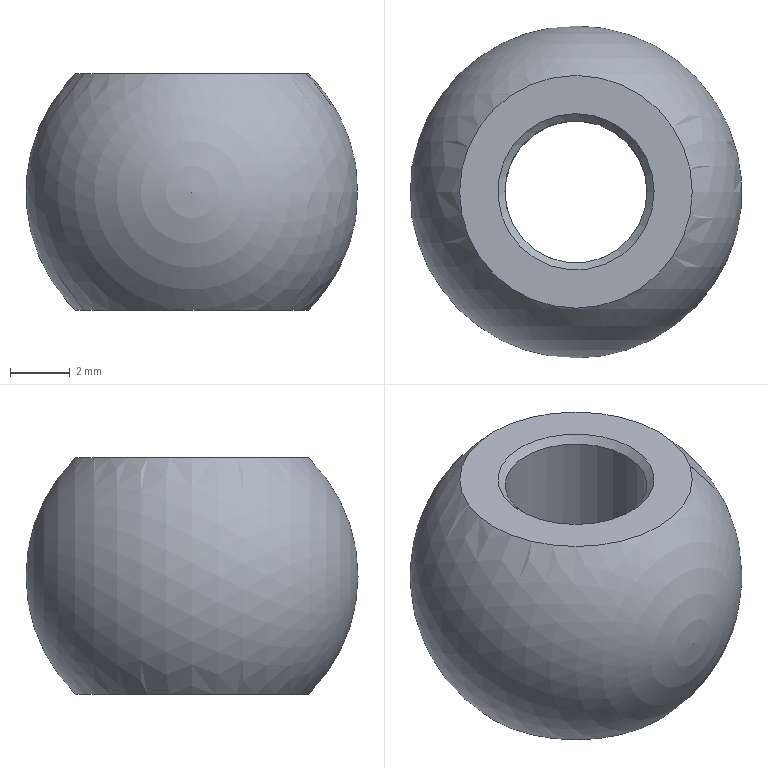Part | NX | features MG0312 tapped 1064K711(1064K711) 2 | 1 solid | 6 faces | box 11.125 x 11.125 x 7.938 mm | volume 498.388 mm3 | plane 2 | cone 2 | sphere 1 | cylinder 1 | commonest cylinder face diameters 4.763 x1
STEP:
#1=CARTESIAN_POINT('',(0.,10.39,-3.969));
#2=VERTEX_POINT('',#1);
#3=CARTESIAN_POINT('',(0.,14.287,-3.969));
#4=DIRECTION('',(0.,0.,1.));
#5=DIRECTION('',(0.,-1.,0.));
#6=AXIS2_PLACEMENT_3D('',#3,#4,#5);
#7=CIRCLE('',#6,3.898);
#8=EDGE_CURVE('',#2,#2,#7,.F.);
#9=ORIENTED_EDGE('',*,*,#8,.F.);
#10=EDGE_LOOP('',(#9));
#11=FACE_BOUND('',#10,.T.);
#12=CARTESIAN_POINT('',(0.,18.185,3.969));
#13=VERTEX_POINT('',#12);
#14=CARTESIAN_POINT('',(0.,14.287,3.969));
#15=DIRECTION('',(0.,0.,-1.));
#16=DIRECTION('',(0.,1.,0.));
#17=AXIS2_PLACEMENT_3D('',#14,#15,#16);
#18=CIRCLE('',#17,3.898);
#19=EDGE_CURVE('',#13,#13,#18,.F.);
#20=ORIENTED_EDGE('',*,*,#19,.F.);
#21=EDGE_LOOP('',(#20));
#22=FACE_BOUND('',#21,.T.);
#23=CARTESIAN_POINT('',(0.,14.287,0.));
#24=DIRECTION('',(0.,-1.,0.));
#25=DIRECTION('',(-1.,0.,0.));
#26=AXIS2_PLACEMENT_3D('',#23,#24,#25);
#27=SPHERICAL_SURFACE('',#26,5.563);
#28=ADVANCED_FACE('',(#11,#22),#27,.T.);
#29=CARTESIAN_POINT('',(0.,16.907,3.969));
#30=VERTEX_POINT('',#29);
#31=CARTESIAN_POINT('',(0.,14.287,3.969));
#32=DIRECTION('',(0.,0.,-1.));
#33=DIRECTION('',(0.,1.,0.));
#34=AXIS2_PLACEMENT_3D('',#31,#32,#33);
#35=CIRCLE('',#34,2.619);
#36=EDGE_CURVE('',#30,#30,#35,.T.);
#37=ORIENTED_EDGE('',*,*,#36,.T.);
#38=EDGE_LOOP('',(#37));
#39=FACE_BOUND('',#38,.T.);
#40=ORIENTED_EDGE('',*,*,#19,.T.);
#41=EDGE_LOOP('',(#40));
#42=FACE_BOUND('',#41,.T.);
#43=CARTESIAN_POINT('',(-7.938,22.225,3.969));
#44=DIRECTION('',(0.,0.,-1.));
#45=DIRECTION('',(0.,1.,0.));
#46=AXIS2_PLACEMENT_3D('',#43,#44,#45);
#47=PLANE('',#46);
#48=ADVANCED_FACE('',(#39,#42),#47,.F.);
#49=CARTESIAN_POINT('',(0.,11.668,-3.969));
#50=VERTEX_POINT('',#49);
#51=CARTESIAN_POINT('',(0.,14.287,-3.969));
#52=DIRECTION('',(0.,0.,1.));
#53=DIRECTION('',(0.,-1.,0.));
#54=AXIS2_PLACEMENT_3D('',#51,#52,#53);
#55=CIRCLE('',#54,2.619);
#56=EDGE_CURVE('',#50,#50,#55,.T.);
#57=ORIENTED_EDGE('',*,*,#56,.T.);
#58=EDGE_LOOP('',(#57));
#59=FACE_BOUND('',#58,.T.);
#60=ORIENTED_EDGE('',*,*,#8,.T.);
#61=EDGE_LOOP('',(#60));
#62=FACE_BOUND('',#61,.T.);
#63=CARTESIAN_POINT('',(-7.938,22.225,-3.969));
#64=DIRECTION('',(0.,0.,1.));
#65=DIRECTION('',(0.,-1.,0.));
#66=AXIS2_PLACEMENT_3D('',#63,#64,#65);
#67=PLANE('',#66);
#68=ADVANCED_FACE('',(#59,#62),#67,.F.);
#69=CARTESIAN_POINT('',(2.381,14.287,-3.731));
#70=VERTEX_POINT('',#69);
#71=CARTESIAN_POINT('',(0.,14.287,-3.731));
#72=DIRECTION('',(0.,0.,1.));
#73=DIRECTION('',(1.,0.,0.));
#74=AXIS2_PLACEMENT_3D('',#71,#72,#73);
#75=CIRCLE('',#74,2.381);
#76=EDGE_CURVE('',#70,#70,#75,.F.);
#77=ORIENTED_EDGE('',*,*,#76,.T.);
#78=EDGE_LOOP('',(#77));
#79=FACE_BOUND('',#78,.T.);
#80=CARTESIAN_POINT('',(-2.381,14.287,3.731));
#81=VERTEX_POINT('',#80);
#82=CARTESIAN_POINT('',(0.,14.287,3.731));
#83=DIRECTION('',(0.,0.,-1.));
#84=DIRECTION('',(-1.,0.,0.));
#85=AXIS2_PLACEMENT_3D('',#82,#83,#84);
#86=CIRCLE('',#85,2.381);
#87=EDGE_CURVE('',#81,#81,#86,.F.);
#88=ORIENTED_EDGE('',*,*,#87,.T.);
#89=EDGE_LOOP('',(#88));
#90=FACE_BOUND('',#89,.T.);
#91=CARTESIAN_POINT('',(0.,14.287,-3.969));
#92=DIRECTION('',(0.,0.,1.));
#93=DIRECTION('',(1.,0.,0.));
#94=AXIS2_PLACEMENT_3D('',#91,#92,#93);
#95=CYLINDRICAL_SURFACE('',#94,2.381);
#96=ADVANCED_FACE('',(#79,#90),#95,.F.);
#97=ORIENTED_EDGE('',*,*,#76,.F.);
#98=EDGE_LOOP('',(#97));
#99=FACE_BOUND('',#98,.T.);
#100=ORIENTED_EDGE('',*,*,#56,.F.);
#101=EDGE_LOOP('',(#100));
#102=FACE_BOUND('',#101,.T.);
#103=CARTESIAN_POINT('',(0.,14.287,-3.969));
#104=DIRECTION('',(0.,0.,-1.));
#105=DIRECTION('',(-1.,0.,0.));
#106=AXIS2_PLACEMENT_3D('',#103,#104,#105);
#107=CONICAL_SURFACE('',#106,2.619,0.7854);
#108=ADVANCED_FACE('',(#99,#102),#107,.F.);
#109=ORIENTED_EDGE('',*,*,#36,.F.);
#110=EDGE_LOOP('',(#109));
#111=FACE_BOUND('',#110,.T.);
#112=ORIENTED_EDGE('',*,*,#87,.F.);
#113=EDGE_LOOP('',(#112));
#114=FACE_BOUND('',#113,.T.);
#115=CARTESIAN_POINT('',(0.,14.287,3.731));
#116=DIRECTION('',(0.,0.,1.));
#117=DIRECTION('',(1.,0.,0.));
#118=AXIS2_PLACEMENT_3D('',#115,#116,#117);
#119=CONICAL_SURFACE('',#118,2.381,0.7854);
#120=ADVANCED_FACE('',(#111,#114),#119,.F.);
#121=CLOSED_SHELL('',(#28,#48,#68,#96,#108,#120));
#122=MANIFOLD_SOLID_BREP('',#121);
#123=(LENGTH_UNIT()NAMED_UNIT(*)SI_UNIT(.MILLI.,.METRE.));
#124=UNCERTAINTY_MEASURE_WITH_UNIT(LENGTH_MEASURE(0.00001),#123,'','');
#125=(NAMED_UNIT(*)PLANE_ANGLE_UNIT()SI_UNIT($,.RADIAN.));
#126=(NAMED_UNIT(*)SI_UNIT($,.STERADIAN.)SOLID_ANGLE_UNIT());
#127=(GEOMETRIC_REPRESENTATION_CONTEXT(3)GLOBAL_UNCERTAINTY_ASSIGNED_CONTEXT((#124))GLOBAL_UNIT_ASSIGNED_CONTEXT((#123,#125,#126))REPRESENTATION_CONTEXT('',''));
#128=ADVANCED_BREP_SHAPE_REPRESENTATION('',(#122),#127);